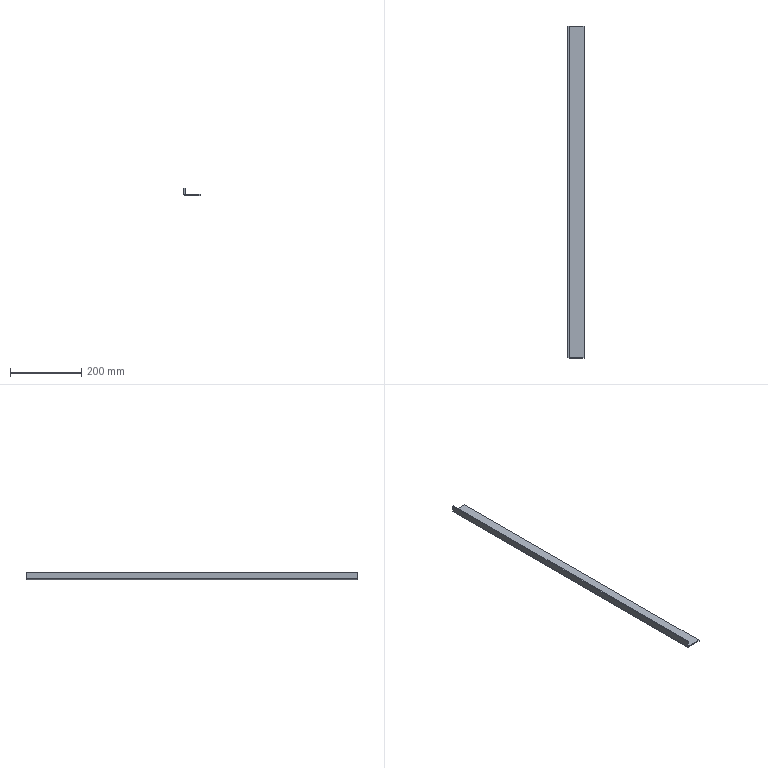Part | STEP file | HESS-408-70-15W-W-8-outer case reinforcing rib 4 | 1 solid | 10 faces | box 45 x 930 x 20 mm | volume 171064 mm3 | plane 8 | cylinder 2 | commonest cylinder face diameters 0.2 x1 6.2 x1
STEP:
#1=CARTESIAN_POINT('',(0.,0.,0.));
#2=DIRECTION('',(0.,0.,1.));
#3=DIRECTION('',(1.,0.,0.));
#4=AXIS2_PLACEMENT_3D('',#1,#2,#3);
#5=CARTESIAN_POINT('',(45.,465.,-17.));
#6=VERTEX_POINT('',#5);
#7=CARTESIAN_POINT('',(45.,-465.,-17.));
#8=VERTEX_POINT('',#7);
#9=CARTESIAN_POINT('',(45.,465.,-17.));
#10=DIRECTION('',(0.,-1.,0.));
#11=VECTOR('',#10,1.);
#12=LINE('',#9,#11);
#13=CARTESIAN_POINT('',(0.,465.,-17.));
#14=DIRECTION('',(0.,0.,-1.));
#15=DIRECTION('',(-1.,0.,0.));
#16=AXIS2_PLACEMENT_3D('',#13,#14,#15);
#17=PLANE('',#16);
#18=CARTESIAN_POINT('',(-45.,0.));
#19=DIRECTION('',(0.,-1.));
#20=VECTOR('',#19,1.);
#21=LINE('',#18,#20);
#22=(GEOMETRIC_REPRESENTATION_CONTEXT(2)PARAMETRIC_REPRESENTATION_CONTEXT()REPRESENTATION_CONTEXT('',''));
#23=DEFINITIONAL_REPRESENTATION('',(#21),#22);
#24=PCURVE('',#17,#23);
#25=CARTESIAN_POINT('',(45.,465.,-20.));
#26=DIRECTION('',(1.,0.,0.));
#27=DIRECTION('',(0.,0.,-1.));
#28=AXIS2_PLACEMENT_3D('',#25,#26,#27);
#29=PLANE('',#28);
#30=CARTESIAN_POINT('',(-3.,0.));
#31=DIRECTION('',(0.,-1.));
#32=VECTOR('',#31,1.);
#33=LINE('',#30,#32);
#34=(GEOMETRIC_REPRESENTATION_CONTEXT(2)PARAMETRIC_REPRESENTATION_CONTEXT()REPRESENTATION_CONTEXT('',''));
#35=DEFINITIONAL_REPRESENTATION('',(#33),#34);
#36=PCURVE('',#29,#35);
#37=SURFACE_CURVE('',#12,(#24,#36),.PCURVE_S1.);
#38=EDGE_CURVE('',#6,#8,#37,.T.);
#39=ORIENTED_EDGE('',*,*,#38,.F.);
#40=CARTESIAN_POINT('',(3.1,465.,-17.));
#41=VERTEX_POINT('',#40);
#42=CARTESIAN_POINT('',(0.,465.,-17.));
#43=DIRECTION('',(1.,0.,0.));
#44=VECTOR('',#43,1.);
#45=LINE('',#42,#44);
#46=CARTESIAN_POINT('',(0.,0.));
#47=DIRECTION('',(-1.,0.));
#48=VECTOR('',#47,1.);
#49=LINE('',#46,#48);
#50=(GEOMETRIC_REPRESENTATION_CONTEXT(2)PARAMETRIC_REPRESENTATION_CONTEXT()REPRESENTATION_CONTEXT('',''));
#51=DEFINITIONAL_REPRESENTATION('',(#49),#50);
#52=PCURVE('',#17,#51);
#53=CARTESIAN_POINT('',(3.,465.,-16.9));
#54=DIRECTION('',(0.,1.,0.));
#55=DIRECTION('',(-1.,0.,0.));
#56=AXIS2_PLACEMENT_3D('',#53,#54,#55);
#57=PLANE('',#56);
#58=CARTESIAN_POINT('',(3.,-0.1));
#59=DIRECTION('',(-1.,0.));
#60=VECTOR('',#59,1.);
#61=LINE('',#58,#60);
#62=(GEOMETRIC_REPRESENTATION_CONTEXT(2)PARAMETRIC_REPRESENTATION_CONTEXT()REPRESENTATION_CONTEXT('',''));
#63=DEFINITIONAL_REPRESENTATION('',(#61),#62);
#64=PCURVE('',#57,#63);
#65=SURFACE_CURVE('',#45,(#52,#64),.PCURVE_S1.);
#66=EDGE_CURVE('',#41,#6,#65,.T.);
#67=ORIENTED_EDGE('',*,*,#66,.F.);
#68=CARTESIAN_POINT('',(3.1,-465.,-17.));
#69=VERTEX_POINT('',#68);
#70=CARTESIAN_POINT('',(3.1,465.,-17.));
#71=DIRECTION('',(0.,1.,0.));
#72=VECTOR('',#71,1.);
#73=LINE('',#70,#72);
#74=CARTESIAN_POINT('',(-3.1,0.));
#75=DIRECTION('',(0.,1.));
#76=VECTOR('',#75,1.);
#77=LINE('',#74,#76);
#78=(GEOMETRIC_REPRESENTATION_CONTEXT(2)PARAMETRIC_REPRESENTATION_CONTEXT()REPRESENTATION_CONTEXT('',''));
#79=DEFINITIONAL_REPRESENTATION('',(#77),#78);
#80=PCURVE('',#17,#79);
#81=CARTESIAN_POINT('',(3.1,465.,-16.9));
#82=DIRECTION('',(0.,-1.,0.));
#83=DIRECTION('',(1.,0.,0.));
#84=AXIS2_PLACEMENT_3D('',#81,#82,#83);
#85=CYLINDRICAL_SURFACE('',#84,0.1);
#86=CARTESIAN_POINT('',(4.712,0.));
#87=DIRECTION('',(0.,-1.));
#88=VECTOR('',#87,1.);
#89=LINE('',#86,#88);
#90=(GEOMETRIC_REPRESENTATION_CONTEXT(2)PARAMETRIC_REPRESENTATION_CONTEXT()REPRESENTATION_CONTEXT('',''));
#91=DEFINITIONAL_REPRESENTATION('',(#89),#90);
#92=PCURVE('',#85,#91);
#93=SURFACE_CURVE('',#73,(#80,#92),.PCURVE_S1.);
#94=EDGE_CURVE('',#69,#41,#93,.T.);
#95=ORIENTED_EDGE('',*,*,#94,.F.);
#96=CARTESIAN_POINT('',(0.,-465.,-17.));
#97=DIRECTION('',(-1.,0.,0.));
#98=VECTOR('',#97,1.);
#99=LINE('',#96,#98);
#100=CARTESIAN_POINT('',(0.,-930.));
#101=DIRECTION('',(1.,0.));
#102=VECTOR('',#101,1.);
#103=LINE('',#100,#102);
#104=(GEOMETRIC_REPRESENTATION_CONTEXT(2)PARAMETRIC_REPRESENTATION_CONTEXT()REPRESENTATION_CONTEXT('',''));
#105=DEFINITIONAL_REPRESENTATION('',(#103),#104);
#106=PCURVE('',#17,#105);
#107=CARTESIAN_POINT('',(3.1,-465.,-16.9));
#108=DIRECTION('',(0.,1.,0.));
#109=DIRECTION('',(-1.,0.,0.));
#110=AXIS2_PLACEMENT_3D('',#107,#108,#109);
#111=PLANE('',#110);
#112=CARTESIAN_POINT('',(3.1,-0.1));
#113=DIRECTION('',(1.,0.));
#114=VECTOR('',#113,1.);
#115=LINE('',#112,#114);
#116=(GEOMETRIC_REPRESENTATION_CONTEXT(2)PARAMETRIC_REPRESENTATION_CONTEXT()REPRESENTATION_CONTEXT('',''));
#117=DEFINITIONAL_REPRESENTATION('',(#115),#116);
#118=PCURVE('',#111,#117);
#119=SURFACE_CURVE('',#99,(#106,#118),.PCURVE_S1.);
#120=EDGE_CURVE('',#8,#69,#119,.T.);
#121=ORIENTED_EDGE('',*,*,#120,.F.);
#122=EDGE_LOOP('',(#39,#67,#95,#121));
#123=FACE_BOUND('',#122,.T.);
#124=ADVANCED_FACE('',(#123),#17,.F.);
#125=ORIENTED_EDGE('',*,*,#120,.T.);
#126=CARTESIAN_POINT('',(3.,-465.,-16.9));
#127=VERTEX_POINT('',#126);
#128=CARTESIAN_POINT('',(3.1,-465.,-16.9));
#129=DIRECTION('',(0.,1.,0.));
#130=DIRECTION('',(1.,0.,0.));
#131=AXIS2_PLACEMENT_3D('',#128,#129,#130);
#132=CIRCLE('',#131,0.1);
#133=CARTESIAN_POINT('',(0.,0.));
#134=DIRECTION('',(-1.,0.));
#135=AXIS2_PLACEMENT_2D('',#133,#134);
#136=CIRCLE('',#135,0.1);
#137=(GEOMETRIC_REPRESENTATION_CONTEXT(2)PARAMETRIC_REPRESENTATION_CONTEXT()REPRESENTATION_CONTEXT('',''));
#138=DEFINITIONAL_REPRESENTATION('',(#136),#137);
#139=PCURVE('',#111,#138);
#140=CARTESIAN_POINT('',(6.283,930.));
#141=DIRECTION('',(-1.,0.));
#142=VECTOR('',#141,1.);
#143=LINE('',#140,#142);
#144=(GEOMETRIC_REPRESENTATION_CONTEXT(2)PARAMETRIC_REPRESENTATION_CONTEXT()REPRESENTATION_CONTEXT('',''));
#145=DEFINITIONAL_REPRESENTATION('',(#143),#144);
#146=PCURVE('',#85,#145);
#147=SURFACE_CURVE('',#132,(#139,#146),.PCURVE_S1.);
#148=EDGE_CURVE('',#69,#127,#147,.T.);
#149=ORIENTED_EDGE('',*,*,#148,.T.);
#150=CARTESIAN_POINT('',(3.,-465.,0.));
#151=VERTEX_POINT('',#150);
#152=CARTESIAN_POINT('',(3.,-465.,0.));
#153=DIRECTION('',(0.,0.,1.));
#154=VECTOR('',#153,1.);
#155=LINE('',#152,#154);
#156=CARTESIAN_POINT('',(0.1,16.9));
#157=DIRECTION('',(0.,1.));
#158=VECTOR('',#157,1.);
#159=LINE('',#156,#158);
#160=(GEOMETRIC_REPRESENTATION_CONTEXT(2)PARAMETRIC_REPRESENTATION_CONTEXT()REPRESENTATION_CONTEXT('',''));
#161=DEFINITIONAL_REPRESENTATION('',(#159),#160);
#162=PCURVE('',#111,#161);
#163=CARTESIAN_POINT('',(3.,465.,0.));
#164=DIRECTION('',(-1.,0.,0.));
#165=DIRECTION('',(0.,0.,1.));
#166=AXIS2_PLACEMENT_3D('',#163,#164,#165);
#167=PLANE('',#166);
#168=CARTESIAN_POINT('',(0.,-930.));
#169=DIRECTION('',(1.,0.));
#170=VECTOR('',#169,1.);
#171=LINE('',#168,#170);
#172=(GEOMETRIC_REPRESENTATION_CONTEXT(2)PARAMETRIC_REPRESENTATION_CONTEXT()REPRESENTATION_CONTEXT('',''));
#173=DEFINITIONAL_REPRESENTATION('',(#171),#172);
#174=PCURVE('',#167,#173);
#175=SURFACE_CURVE('',#155,(#162,#174),.PCURVE_S1.);
#176=EDGE_CURVE('',#127,#151,#175,.T.);
#177=ORIENTED_EDGE('',*,*,#176,.T.);
#178=CARTESIAN_POINT('',(0.,-465.,0.));
#179=VERTEX_POINT('',#178);
#180=CARTESIAN_POINT('',(3.1,-465.,0.));
#181=DIRECTION('',(-1.,0.,0.));
#182=VECTOR('',#181,1.);
#183=LINE('',#180,#182);
#184=CARTESIAN_POINT('',(0.,16.9));
#185=DIRECTION('',(1.,0.));
#186=VECTOR('',#185,1.);
#187=LINE('',#184,#186);
#188=(GEOMETRIC_REPRESENTATION_CONTEXT(2)PARAMETRIC_REPRESENTATION_CONTEXT()REPRESENTATION_CONTEXT('',''));
#189=DEFINITIONAL_REPRESENTATION('',(#187),#188);
#190=PCURVE('',#111,#189);
#191=CARTESIAN_POINT('',(3.,465.,0.));
#192=DIRECTION('',(0.,0.,1.));
#193=DIRECTION('',(1.,0.,0.));
#194=AXIS2_PLACEMENT_3D('',#191,#192,#193);
#195=PLANE('',#194);
#196=CARTESIAN_POINT('',(0.1,-930.));
#197=DIRECTION('',(-1.,0.));
#198=VECTOR('',#197,1.);
#199=LINE('',#196,#198);
#200=(GEOMETRIC_REPRESENTATION_CONTEXT(2)PARAMETRIC_REPRESENTATION_CONTEXT()REPRESENTATION_CONTEXT('',''));
#201=DEFINITIONAL_REPRESENTATION('',(#199),#200);
#202=PCURVE('',#195,#201);
#203=SURFACE_CURVE('',#183,(#190,#202),.PCURVE_S1.);
#204=EDGE_CURVE('',#151,#179,#203,.T.);
#205=ORIENTED_EDGE('',*,*,#204,.T.);
#206=CARTESIAN_POINT('',(0.,-465.,-16.9));
#207=VERTEX_POINT('',#206);
#208=CARTESIAN_POINT('',(0.,-465.,-17.));
#209=DIRECTION('',(0.,0.,-1.));
#210=VECTOR('',#209,1.);
#211=LINE('',#208,#210);
#212=CARTESIAN_POINT('',(3.1,-0.1));
#213=DIRECTION('',(0.,-1.));
#214=VECTOR('',#213,1.);
#215=LINE('',#212,#214);
#216=(GEOMETRIC_REPRESENTATION_CONTEXT(2)PARAMETRIC_REPRESENTATION_CONTEXT()REPRESENTATION_CONTEXT('',''));
#217=DEFINITIONAL_REPRESENTATION('',(#215),#216);
#218=PCURVE('',#111,#217);
#219=CARTESIAN_POINT('',(0.,465.,0.));
#220=DIRECTION('',(-1.,0.,0.));
#221=DIRECTION('',(0.,0.,1.));
#222=AXIS2_PLACEMENT_3D('',#219,#220,#221);
#223=PLANE('',#222);
#224=CARTESIAN_POINT('',(-17.,-930.));
#225=DIRECTION('',(-1.,0.));
#226=VECTOR('',#225,1.);
#227=LINE('',#224,#226);
#228=(GEOMETRIC_REPRESENTATION_CONTEXT(2)PARAMETRIC_REPRESENTATION_CONTEXT()REPRESENTATION_CONTEXT('',''));
#229=DEFINITIONAL_REPRESENTATION('',(#227),#228);
#230=PCURVE('',#223,#229);
#231=SURFACE_CURVE('',#211,(#218,#230),.PCURVE_S1.);
#232=EDGE_CURVE('',#179,#207,#231,.T.);
#233=ORIENTED_EDGE('',*,*,#232,.T.);
#234=CARTESIAN_POINT('',(3.1,-465.,-20.));
#235=VERTEX_POINT('',#234);
#236=CARTESIAN_POINT('',(3.1,-465.,-16.9));
#237=DIRECTION('',(0.,-1.,0.));
#238=DIRECTION('',(1.,0.,0.));
#239=AXIS2_PLACEMENT_3D('',#236,#237,#238);
#240=CIRCLE('',#239,3.1);
#241=CARTESIAN_POINT('',(-3.1,0.));
#242=CARTESIAN_POINT('',(-3.1,5.369));
#243=CARTESIAN_POINT('',(1.55,2.685));
#244=CARTESIAN_POINT('',(6.2,0.));
#245=CARTESIAN_POINT('',(1.55,-2.685));
#246=CARTESIAN_POINT('',(-3.1,-5.369));
#247=CARTESIAN_POINT('',(-3.1,0.));
#248=(BOUNDED_CURVE()B_SPLINE_CURVE(2,(#241,#242,#243,#244,#245,#246,#247),.UNSPECIFIED.,.T.,.F.)B_SPLINE_CURVE_WITH_KNOTS((1,2,2,2,2,1),(-2.094,0.,2.094,4.189,6.283,8.378),.UNSPECIFIED.)CURVE()GEOMETRIC_REPRESENTATION_ITEM()RATIONAL_B_SPLINE_CURVE((1.,0.5,1.,0.5,1.,0.5,1.))REPRESENTATION_ITEM(''));
#249=(GEOMETRIC_REPRESENTATION_CONTEXT(2)PARAMETRIC_REPRESENTATION_CONTEXT()REPRESENTATION_CONTEXT('',''));
#250=DEFINITIONAL_REPRESENTATION('',(#248),#249);
#251=PCURVE('',#111,#250);
#252=CARTESIAN_POINT('',(3.1,465.,-16.9));
#253=DIRECTION('',(0.,-1.,0.));
#254=DIRECTION('',(1.,0.,0.));
#255=AXIS2_PLACEMENT_3D('',#252,#253,#254);
#256=CYLINDRICAL_SURFACE('',#255,3.1);
#257=CARTESIAN_POINT('',(0.,930.));
#258=DIRECTION('',(1.,0.));
#259=VECTOR('',#258,1.);
#260=LINE('',#257,#259);
#261=(GEOMETRIC_REPRESENTATION_CONTEXT(2)PARAMETRIC_REPRESENTATION_CONTEXT()REPRESENTATION_CONTEXT('',''));
#262=DEFINITIONAL_REPRESENTATION('',(#260),#261);
#263=PCURVE('',#256,#262);
#264=SURFACE_CURVE('',#240,(#251,#263),.PCURVE_S1.);
#265=EDGE_CURVE('',#207,#235,#264,.T.);
#266=ORIENTED_EDGE('',*,*,#265,.T.);
#267=CARTESIAN_POINT('',(45.,-465.,-20.));
#268=VERTEX_POINT('',#267);
#269=CARTESIAN_POINT('',(3.1,-465.,-20.));
#270=DIRECTION('',(-1.,0.,0.));
#271=VECTOR('',#270,1.);
#272=LINE('',#269,#271);
#273=CARTESIAN_POINT('',(0.,-3.1));
#274=DIRECTION('',(1.,0.));
#275=VECTOR('',#274,1.);
#276=LINE('',#273,#275);
#277=(GEOMETRIC_REPRESENTATION_CONTEXT(2)PARAMETRIC_REPRESENTATION_CONTEXT()REPRESENTATION_CONTEXT('',''));
#278=DEFINITIONAL_REPRESENTATION('',(#276),#277);
#279=PCURVE('',#111,#278);
#280=CARTESIAN_POINT('',(0.,465.,-20.));
#281=DIRECTION('',(0.,0.,-1.));
#282=DIRECTION('',(-1.,0.,0.));
#283=AXIS2_PLACEMENT_3D('',#280,#281,#282);
#284=PLANE('',#283);
#285=CARTESIAN_POINT('',(-3.1,-930.));
#286=DIRECTION('',(1.,0.));
#287=VECTOR('',#286,1.);
#288=LINE('',#285,#287);
#289=(GEOMETRIC_REPRESENTATION_CONTEXT(2)PARAMETRIC_REPRESENTATION_CONTEXT()REPRESENTATION_CONTEXT('',''));
#290=DEFINITIONAL_REPRESENTATION('',(#288),#289);
#291=PCURVE('',#284,#290);
#292=SURFACE_CURVE('',#272,(#279,#291),.PCURVE_S1.);
#293=EDGE_CURVE('',#268,#235,#292,.T.);
#294=ORIENTED_EDGE('',*,*,#293,.F.);
#295=CARTESIAN_POINT('',(45.,-465.,-16.9));
#296=DIRECTION('',(0.,0.,-1.));
#297=VECTOR('',#296,1.);
#298=LINE('',#295,#297);
#299=CARTESIAN_POINT('',(-41.9,0.));
#300=DIRECTION('',(0.,-1.));
#301=VECTOR('',#300,1.);
#302=LINE('',#299,#301);
#303=(GEOMETRIC_REPRESENTATION_CONTEXT(2)PARAMETRIC_REPRESENTATION_CONTEXT()REPRESENTATION_CONTEXT('',''));
#304=DEFINITIONAL_REPRESENTATION('',(#302),#303);
#305=PCURVE('',#111,#304);
#306=CARTESIAN_POINT('',(-3.1,-930.));
#307=DIRECTION('',(1.,0.));
#308=VECTOR('',#307,1.);
#309=LINE('',#306,#308);
#310=(GEOMETRIC_REPRESENTATION_CONTEXT(2)PARAMETRIC_REPRESENTATION_CONTEXT()REPRESENTATION_CONTEXT('',''));
#311=DEFINITIONAL_REPRESENTATION('',(#309),#310);
#312=PCURVE('',#29,#311);
#313=SURFACE_CURVE('',#298,(#305,#312),.PCURVE_S1.);
#314=EDGE_CURVE('',#8,#268,#313,.T.);
#315=ORIENTED_EDGE('',*,*,#314,.F.);
#316=EDGE_LOOP('',(#125,#149,#177,#205,#233,#266,#294,#315));
#317=FACE_BOUND('',#316,.T.);
#318=ADVANCED_FACE('',(#317),#111,.F.);
#319=CARTESIAN_POINT('',(45.,465.,-20.));
#320=VERTEX_POINT('',#319);
#321=CARTESIAN_POINT('',(45.,465.,-20.));
#322=DIRECTION('',(0.,0.,1.));
#323=VECTOR('',#322,1.);
#324=LINE('',#321,#323);
#325=CARTESIAN_POINT('',(0.,0.));
#326=DIRECTION('',(-1.,0.));
#327=VECTOR('',#326,1.);
#328=LINE('',#325,#327);
#329=(GEOMETRIC_REPRESENTATION_CONTEXT(2)PARAMETRIC_REPRESENTATION_CONTEXT()REPRESENTATION_CONTEXT('',''));
#330=DEFINITIONAL_REPRESENTATION('',(#328),#329);
#331=PCURVE('',#29,#330);
#332=CARTESIAN_POINT('',(-42.,-3.1));
#333=DIRECTION('',(0.,1.));
#334=VECTOR('',#333,1.);
#335=LINE('',#332,#334);
#336=(GEOMETRIC_REPRESENTATION_CONTEXT(2)PARAMETRIC_REPRESENTATION_CONTEXT()REPRESENTATION_CONTEXT('',''));
#337=DEFINITIONAL_REPRESENTATION('',(#335),#336);
#338=PCURVE('',#57,#337);
#339=SURFACE_CURVE('',#324,(#331,#338),.PCURVE_S1.);
#340=EDGE_CURVE('',#320,#6,#339,.T.);
#341=ORIENTED_EDGE('',*,*,#340,.T.);
#342=ORIENTED_EDGE('',*,*,#38,.T.);
#343=ORIENTED_EDGE('',*,*,#314,.T.);
#344=CARTESIAN_POINT('',(45.,465.,-20.));
#345=DIRECTION('',(0.,1.,0.));
#346=VECTOR('',#345,1.);
#347=LINE('',#344,#346);
#348=CARTESIAN_POINT('',(0.,0.));
#349=DIRECTION('',(0.,1.));
#350=VECTOR('',#349,1.);
#351=LINE('',#348,#350);
#352=(GEOMETRIC_REPRESENTATION_CONTEXT(2)PARAMETRIC_REPRESENTATION_CONTEXT()REPRESENTATION_CONTEXT('',''));
#353=DEFINITIONAL_REPRESENTATION('',(#351),#352);
#354=PCURVE('',#29,#353);
#355=CARTESIAN_POINT('',(-45.,0.));
#356=DIRECTION('',(0.,1.));
#357=VECTOR('',#356,1.);
#358=LINE('',#355,#357);
#359=(GEOMETRIC_REPRESENTATION_CONTEXT(2)PARAMETRIC_REPRESENTATION_CONTEXT()REPRESENTATION_CONTEXT('',''));
#360=DEFINITIONAL_REPRESENTATION('',(#358),#359);
#361=PCURVE('',#284,#360);
#362=SURFACE_CURVE('',#347,(#354,#361),.PCURVE_S1.);
#363=EDGE_CURVE('',#268,#320,#362,.T.);
#364=ORIENTED_EDGE('',*,*,#363,.T.);
#365=EDGE_LOOP('',(#341,#342,#343,#364));
#366=FACE_BOUND('',#365,.T.);
#367=ADVANCED_FACE('',(#366),#29,.T.);
#368=ORIENTED_EDGE('',*,*,#66,.T.);
#369=ORIENTED_EDGE('',*,*,#340,.F.);
#370=CARTESIAN_POINT('',(3.1,465.,-20.));
#371=VERTEX_POINT('',#370);
#372=CARTESIAN_POINT('',(3.,465.,-20.));
#373=DIRECTION('',(-1.,0.,0.));
#374=VECTOR('',#373,1.);
#375=LINE('',#372,#374);
#376=CARTESIAN_POINT('',(0.,-3.1));
#377=DIRECTION('',(1.,0.));
#378=VECTOR('',#377,1.);
#379=LINE('',#376,#378);
#380=(GEOMETRIC_REPRESENTATION_CONTEXT(2)PARAMETRIC_REPRESENTATION_CONTEXT()REPRESENTATION_CONTEXT('',''));
#381=DEFINITIONAL_REPRESENTATION('',(#379),#380);
#382=PCURVE('',#57,#381);
#383=CARTESIAN_POINT('',(-3.,0.));
#384=DIRECTION('',(1.,0.));
#385=VECTOR('',#384,1.);
#386=LINE('',#383,#385);
#387=(GEOMETRIC_REPRESENTATION_CONTEXT(2)PARAMETRIC_REPRESENTATION_CONTEXT()REPRESENTATION_CONTEXT('',''));
#388=DEFINITIONAL_REPRESENTATION('',(#386),#387);
#389=PCURVE('',#284,#388);
#390=SURFACE_CURVE('',#375,(#382,#389),.PCURVE_S1.);
#391=EDGE_CURVE('',#320,#371,#390,.T.);
#392=ORIENTED_EDGE('',*,*,#391,.T.);
#393=CARTESIAN_POINT('',(0.,465.,-16.9));
#394=VERTEX_POINT('',#393);
#395=CARTESIAN_POINT('',(3.1,465.,-16.9));
#396=DIRECTION('',(0.,1.,0.));
#397=DIRECTION('',(1.,0.,0.));
#398=AXIS2_PLACEMENT_3D('',#395,#396,#397);
#399=CIRCLE('',#398,3.1);
#400=CARTESIAN_POINT('',(-0.1,0.));
#401=DIRECTION('',(-1.,0.));
#402=AXIS2_PLACEMENT_2D('',#400,#401);
#403=CIRCLE('',#402,3.1);
#404=(GEOMETRIC_REPRESENTATION_CONTEXT(2)PARAMETRIC_REPRESENTATION_CONTEXT()REPRESENTATION_CONTEXT('',''));
#405=DEFINITIONAL_REPRESENTATION('',(#403),#404);
#406=PCURVE('',#57,#405);
#407=CARTESIAN_POINT('',(6.283,0.));
#408=DIRECTION('',(-1.,0.));
#409=VECTOR('',#408,1.);
#410=LINE('',#407,#409);
#411=(GEOMETRIC_REPRESENTATION_CONTEXT(2)PARAMETRIC_REPRESENTATION_CONTEXT()REPRESENTATION_CONTEXT('',''));
#412=DEFINITIONAL_REPRESENTATION('',(#410),#411);
#413=PCURVE('',#256,#412);
#414=SURFACE_CURVE('',#399,(#406,#413),.PCURVE_S1.);
#415=EDGE_CURVE('',#371,#394,#414,.T.);
#416=ORIENTED_EDGE('',*,*,#415,.T.);
#417=CARTESIAN_POINT('',(0.,465.,0.));
#418=VERTEX_POINT('',#417);
#419=CARTESIAN_POINT('',(0.,465.,-16.9));
#420=DIRECTION('',(0.,0.,1.));
#421=VECTOR('',#420,1.);
#422=LINE('',#419,#421);
#423=CARTESIAN_POINT('',(3.,0.));
#424=DIRECTION('',(0.,1.));
#425=VECTOR('',#424,1.);
#426=LINE('',#423,#425);
#427=(GEOMETRIC_REPRESENTATION_CONTEXT(2)PARAMETRIC_REPRESENTATION_CONTEXT()REPRESENTATION_CONTEXT('',''));
#428=DEFINITIONAL_REPRESENTATION('',(#426),#427);
#429=PCURVE('',#57,#428);
#430=CARTESIAN_POINT('',(-16.9,0.));
#431=DIRECTION('',(1.,0.));
#432=VECTOR('',#431,1.);
#433=LINE('',#430,#432);
#434=(GEOMETRIC_REPRESENTATION_CONTEXT(2)PARAMETRIC_REPRESENTATION_CONTEXT()REPRESENTATION_CONTEXT('',''));
#435=DEFINITIONAL_REPRESENTATION('',(#433),#434);
#436=PCURVE('',#223,#435);
#437=SURFACE_CURVE('',#422,(#429,#436),.PCURVE_S1.);
#438=EDGE_CURVE('',#394,#418,#437,.T.);
#439=ORIENTED_EDGE('',*,*,#438,.T.);
#440=CARTESIAN_POINT('',(3.,465.,0.));
#441=VERTEX_POINT('',#440);
#442=CARTESIAN_POINT('',(3.1,465.,0.));
#443=DIRECTION('',(1.,0.,0.));
#444=VECTOR('',#443,1.);
#445=LINE('',#442,#444);
#446=CARTESIAN_POINT('',(-0.1,16.9));
#447=DIRECTION('',(-1.,0.));
#448=VECTOR('',#447,1.);
#449=LINE('',#446,#448);
#450=(GEOMETRIC_REPRESENTATION_CONTEXT(2)PARAMETRIC_REPRESENTATION_CONTEXT()REPRESENTATION_CONTEXT('',''));
#451=DEFINITIONAL_REPRESENTATION('',(#449),#450);
#452=PCURVE('',#57,#451);
#453=CARTESIAN_POINT('',(0.1,0.));
#454=DIRECTION('',(1.,0.));
#455=VECTOR('',#454,1.);
#456=LINE('',#453,#455);
#457=(GEOMETRIC_REPRESENTATION_CONTEXT(2)PARAMETRIC_REPRESENTATION_CONTEXT()REPRESENTATION_CONTEXT('',''));
#458=DEFINITIONAL_REPRESENTATION('',(#456),#457);
#459=PCURVE('',#195,#458);
#460=SURFACE_CURVE('',#445,(#452,#459),.PCURVE_S1.);
#461=EDGE_CURVE('',#418,#441,#460,.T.);
#462=ORIENTED_EDGE('',*,*,#461,.T.);
#463=CARTESIAN_POINT('',(3.,465.,-16.9));
#464=VERTEX_POINT('',#463);
#465=CARTESIAN_POINT('',(3.,465.,0.));
#466=DIRECTION('',(0.,0.,-1.));
#467=VECTOR('',#466,1.);
#468=LINE('',#465,#467);
#469=CARTESIAN_POINT('',(0.,16.9));
#470=DIRECTION('',(0.,-1.));
#471=VECTOR('',#470,1.);
#472=LINE('',#469,#471);
#473=(GEOMETRIC_REPRESENTATION_CONTEXT(2)PARAMETRIC_REPRESENTATION_CONTEXT()REPRESENTATION_CONTEXT('',''));
#474=DEFINITIONAL_REPRESENTATION('',(#472),#473);
#475=PCURVE('',#57,#474);
#476=CARTESIAN_POINT('',(0.,0.));
#477=DIRECTION('',(-1.,0.));
#478=VECTOR('',#477,1.);
#479=LINE('',#476,#478);
#480=(GEOMETRIC_REPRESENTATION_CONTEXT(2)PARAMETRIC_REPRESENTATION_CONTEXT()REPRESENTATION_CONTEXT('',''));
#481=DEFINITIONAL_REPRESENTATION('',(#479),#480);
#482=PCURVE('',#167,#481);
#483=SURFACE_CURVE('',#468,(#475,#482),.PCURVE_S1.);
#484=EDGE_CURVE('',#441,#464,#483,.T.);
#485=ORIENTED_EDGE('',*,*,#484,.T.);
#486=CARTESIAN_POINT('',(3.1,465.,-16.9));
#487=DIRECTION('',(0.,-1.,0.));
#488=DIRECTION('',(1.,0.,0.));
#489=AXIS2_PLACEMENT_3D('',#486,#487,#488);
#490=CIRCLE('',#489,0.1);
#491=CARTESIAN_POINT('',(-0.2,0.));
#492=CARTESIAN_POINT('',(-0.2,0.1732));
#493=CARTESIAN_POINT('',(-0.05,0.0866));
#494=CARTESIAN_POINT('',(0.1,0.));
#495=CARTESIAN_POINT('',(-0.05,-0.0866));
#496=CARTESIAN_POINT('',(-0.2,-0.1732));
#497=CARTESIAN_POINT('',(-0.2,0.));
#498=(BOUNDED_CURVE()B_SPLINE_CURVE(2,(#491,#492,#493,#494,#495,#496,#497),.UNSPECIFIED.,.T.,.F.)B_SPLINE_CURVE_WITH_KNOTS((1,2,2,2,2,1),(-2.094,0.,2.094,4.189,6.283,8.378),.UNSPECIFIED.)CURVE()GEOMETRIC_REPRESENTATION_ITEM()RATIONAL_B_SPLINE_CURVE((1.,0.5,1.,0.5,1.,0.5,1.))REPRESENTATION_ITEM(''));
#499=(GEOMETRIC_REPRESENTATION_CONTEXT(2)PARAMETRIC_REPRESENTATION_CONTEXT()REPRESENTATION_CONTEXT('',''));
#500=DEFINITIONAL_REPRESENTATION('',(#498),#499);
#501=PCURVE('',#57,#500);
#502=CARTESIAN_POINT('',(0.,0.));
#503=DIRECTION('',(1.,0.));
#504=VECTOR('',#503,1.);
#505=LINE('',#502,#504);
#506=(GEOMETRIC_REPRESENTATION_CONTEXT(2)PARAMETRIC_REPRESENTATION_CONTEXT()REPRESENTATION_CONTEXT('',''));
#507=DEFINITIONAL_REPRESENTATION('',(#505),#506);
#508=PCURVE('',#85,#507);
#509=SURFACE_CURVE('',#490,(#501,#508),.PCURVE_S1.);
#510=EDGE_CURVE('',#464,#41,#509,.T.);
#511=ORIENTED_EDGE('',*,*,#510,.T.);
#512=EDGE_LOOP('',(#368,#369,#392,#416,#439,#462,#485,#511));
#513=FACE_BOUND('',#512,.T.);
#514=ADVANCED_FACE('',(#513),#57,.T.);
#515=ORIENTED_EDGE('',*,*,#148,.T.);
#516=CARTESIAN_POINT('',(3.,465.,-16.9));
#517=DIRECTION('',(0.,1.,0.));
#518=VECTOR('',#517,1.);
#519=LINE('',#516,#518);
#520=CARTESIAN_POINT('',(3.142,0.));
#521=DIRECTION('',(0.,-1.));
#522=VECTOR('',#521,1.);
#523=LINE('',#520,#522);
#524=(GEOMETRIC_REPRESENTATION_CONTEXT(2)PARAMETRIC_REPRESENTATION_CONTEXT()REPRESENTATION_CONTEXT('',''));
#525=DEFINITIONAL_REPRESENTATION('',(#523),#524);
#526=PCURVE('',#85,#525);
#527=CARTESIAN_POINT('',(-16.9,0.));
#528=DIRECTION('',(0.,1.));
#529=VECTOR('',#528,1.);
#530=LINE('',#527,#529);
#531=(GEOMETRIC_REPRESENTATION_CONTEXT(2)PARAMETRIC_REPRESENTATION_CONTEXT()REPRESENTATION_CONTEXT('',''));
#532=DEFINITIONAL_REPRESENTATION('',(#530),#531);
#533=PCURVE('',#167,#532);
#534=SURFACE_CURVE('',#519,(#526,#533),.PCURVE_S1.);
#535=EDGE_CURVE('',#127,#464,#534,.T.);
#536=ORIENTED_EDGE('',*,*,#535,.T.);
#537=ORIENTED_EDGE('',*,*,#510,.T.);
#538=ORIENTED_EDGE('',*,*,#94,.F.);
#539=EDGE_LOOP('',(#515,#536,#537,#538));
#540=FACE_BOUND('',#539,.F.);
#541=ADVANCED_FACE('',(#540),#85,.F.);
#542=ORIENTED_EDGE('',*,*,#391,.F.);
#543=ORIENTED_EDGE('',*,*,#363,.F.);
#544=ORIENTED_EDGE('',*,*,#293,.T.);
#545=CARTESIAN_POINT('',(3.1,465.,-20.));
#546=DIRECTION('',(0.,1.,0.));
#547=VECTOR('',#546,1.);
#548=LINE('',#545,#547);
#549=CARTESIAN_POINT('',(-3.1,0.));
#550=DIRECTION('',(0.,1.));
#551=VECTOR('',#550,1.);
#552=LINE('',#549,#551);
#553=(GEOMETRIC_REPRESENTATION_CONTEXT(2)PARAMETRIC_REPRESENTATION_CONTEXT()REPRESENTATION_CONTEXT('',''));
#554=DEFINITIONAL_REPRESENTATION('',(#552),#553);
#555=PCURVE('',#284,#554);
#556=CARTESIAN_POINT('',(4.712,0.));
#557=DIRECTION('',(0.,-1.));
#558=VECTOR('',#557,1.);
#559=LINE('',#556,#558);
#560=(GEOMETRIC_REPRESENTATION_CONTEXT(2)PARAMETRIC_REPRESENTATION_CONTEXT()REPRESENTATION_CONTEXT('',''));
#561=DEFINITIONAL_REPRESENTATION('',(#559),#560);
#562=PCURVE('',#256,#561);
#563=SURFACE_CURVE('',#548,(#555,#562),.PCURVE_S1.);
#564=EDGE_CURVE('',#235,#371,#563,.T.);
#565=ORIENTED_EDGE('',*,*,#564,.T.);
#566=EDGE_LOOP('',(#542,#543,#544,#565));
#567=FACE_BOUND('',#566,.T.);
#568=ADVANCED_FACE('',(#567),#284,.T.);
#569=ORIENTED_EDGE('',*,*,#535,.T.);
#570=ORIENTED_EDGE('',*,*,#484,.F.);
#571=CARTESIAN_POINT('',(3.,465.,0.));
#572=DIRECTION('',(0.,1.,0.));
#573=VECTOR('',#572,1.);
#574=LINE('',#571,#573);
#575=CARTESIAN_POINT('',(0.,0.));
#576=DIRECTION('',(0.,1.));
#577=VECTOR('',#576,1.);
#578=LINE('',#575,#577);
#579=(GEOMETRIC_REPRESENTATION_CONTEXT(2)PARAMETRIC_REPRESENTATION_CONTEXT()REPRESENTATION_CONTEXT('',''));
#580=DEFINITIONAL_REPRESENTATION('',(#578),#579);
#581=PCURVE('',#167,#580);
#582=CARTESIAN_POINT('',(0.,0.));
#583=DIRECTION('',(0.,1.));
#584=VECTOR('',#583,1.);
#585=LINE('',#582,#584);
#586=(GEOMETRIC_REPRESENTATION_CONTEXT(2)PARAMETRIC_REPRESENTATION_CONTEXT()REPRESENTATION_CONTEXT('',''));
#587=DEFINITIONAL_REPRESENTATION('',(#585),#586);
#588=PCURVE('',#195,#587);
#589=SURFACE_CURVE('',#574,(#581,#588),.PCURVE_S1.);
#590=EDGE_CURVE('',#151,#441,#589,.T.);
#591=ORIENTED_EDGE('',*,*,#590,.F.);
#592=ORIENTED_EDGE('',*,*,#176,.F.);
#593=EDGE_LOOP('',(#569,#570,#591,#592));
#594=FACE_BOUND('',#593,.T.);
#595=ADVANCED_FACE('',(#594),#167,.F.);
#596=ORIENTED_EDGE('',*,*,#415,.F.);
#597=ORIENTED_EDGE('',*,*,#564,.F.);
#598=ORIENTED_EDGE('',*,*,#265,.F.);
#599=CARTESIAN_POINT('',(0.,465.,-16.9));
#600=DIRECTION('',(0.,1.,0.));
#601=VECTOR('',#600,1.);
#602=LINE('',#599,#601);
#603=CARTESIAN_POINT('',(3.142,0.));
#604=DIRECTION('',(0.,-1.));
#605=VECTOR('',#604,1.);
#606=LINE('',#603,#605);
#607=(GEOMETRIC_REPRESENTATION_CONTEXT(2)PARAMETRIC_REPRESENTATION_CONTEXT()REPRESENTATION_CONTEXT('',''));
#608=DEFINITIONAL_REPRESENTATION('',(#606),#607);
#609=PCURVE('',#256,#608);
#610=CARTESIAN_POINT('',(-16.9,0.));
#611=DIRECTION('',(0.,1.));
#612=VECTOR('',#611,1.);
#613=LINE('',#610,#612);
#614=(GEOMETRIC_REPRESENTATION_CONTEXT(2)PARAMETRIC_REPRESENTATION_CONTEXT()REPRESENTATION_CONTEXT('',''));
#615=DEFINITIONAL_REPRESENTATION('',(#613),#614);
#616=PCURVE('',#223,#615);
#617=SURFACE_CURVE('',#602,(#609,#616),.PCURVE_S1.);
#618=EDGE_CURVE('',#207,#394,#617,.T.);
#619=ORIENTED_EDGE('',*,*,#618,.T.);
#620=EDGE_LOOP('',(#596,#597,#598,#619));
#621=FACE_BOUND('',#620,.T.);
#622=ADVANCED_FACE('',(#621),#256,.T.);
#623=ORIENTED_EDGE('',*,*,#461,.F.);
#624=CARTESIAN_POINT('',(0.,465.,0.));
#625=DIRECTION('',(0.,-1.,0.));
#626=VECTOR('',#625,1.);
#627=LINE('',#624,#626);
#628=CARTESIAN_POINT('',(-3.,0.));
#629=DIRECTION('',(0.,-1.));
#630=VECTOR('',#629,1.);
#631=LINE('',#628,#630);
#632=(GEOMETRIC_REPRESENTATION_CONTEXT(2)PARAMETRIC_REPRESENTATION_CONTEXT()REPRESENTATION_CONTEXT('',''));
#633=DEFINITIONAL_REPRESENTATION('',(#631),#632);
#634=PCURVE('',#195,#633);
#635=CARTESIAN_POINT('',(0.,0.));
#636=DIRECTION('',(0.,-1.));
#637=VECTOR('',#636,1.);
#638=LINE('',#635,#637);
#639=(GEOMETRIC_REPRESENTATION_CONTEXT(2)PARAMETRIC_REPRESENTATION_CONTEXT()REPRESENTATION_CONTEXT('',''));
#640=DEFINITIONAL_REPRESENTATION('',(#638),#639);
#641=PCURVE('',#223,#640);
#642=SURFACE_CURVE('',#627,(#634,#641),.PCURVE_S1.);
#643=EDGE_CURVE('',#418,#179,#642,.T.);
#644=ORIENTED_EDGE('',*,*,#643,.T.);
#645=ORIENTED_EDGE('',*,*,#204,.F.);
#646=ORIENTED_EDGE('',*,*,#590,.T.);
#647=EDGE_LOOP('',(#623,#644,#645,#646));
#648=FACE_BOUND('',#647,.T.);
#649=ADVANCED_FACE('',(#648),#195,.T.);
#650=ORIENTED_EDGE('',*,*,#438,.F.);
#651=ORIENTED_EDGE('',*,*,#618,.F.);
#652=ORIENTED_EDGE('',*,*,#232,.F.);
#653=ORIENTED_EDGE('',*,*,#643,.F.);
#654=EDGE_LOOP('',(#650,#651,#652,#653));
#655=FACE_BOUND('',#654,.T.);
#656=ADVANCED_FACE('',(#655),#223,.T.);
#657=CLOSED_SHELL('',(#124,#318,#367,#514,#541,#568,#595,#622,#649,#656));
#658=MANIFOLD_SOLID_BREP('',#657);
#659=(LENGTH_UNIT()NAMED_UNIT(*)SI_UNIT(.MILLI.,.METRE.));
#660=UNCERTAINTY_MEASURE_WITH_UNIT(LENGTH_MEASURE(0.0000001),#659,'','');
#661=(NAMED_UNIT(*)PLANE_ANGLE_UNIT()SI_UNIT($,.RADIAN.));
#662=(NAMED_UNIT(*)SI_UNIT($,.STERADIAN.)SOLID_ANGLE_UNIT());
#663=(GEOMETRIC_REPRESENTATION_CONTEXT(3)GLOBAL_UNCERTAINTY_ASSIGNED_CONTEXT((#660))GLOBAL_UNIT_ASSIGNED_CONTEXT((#659,#661,#662))REPRESENTATION_CONTEXT('',''));
#664=ADVANCED_BREP_SHAPE_REPRESENTATION('',(#4,#658),#663);